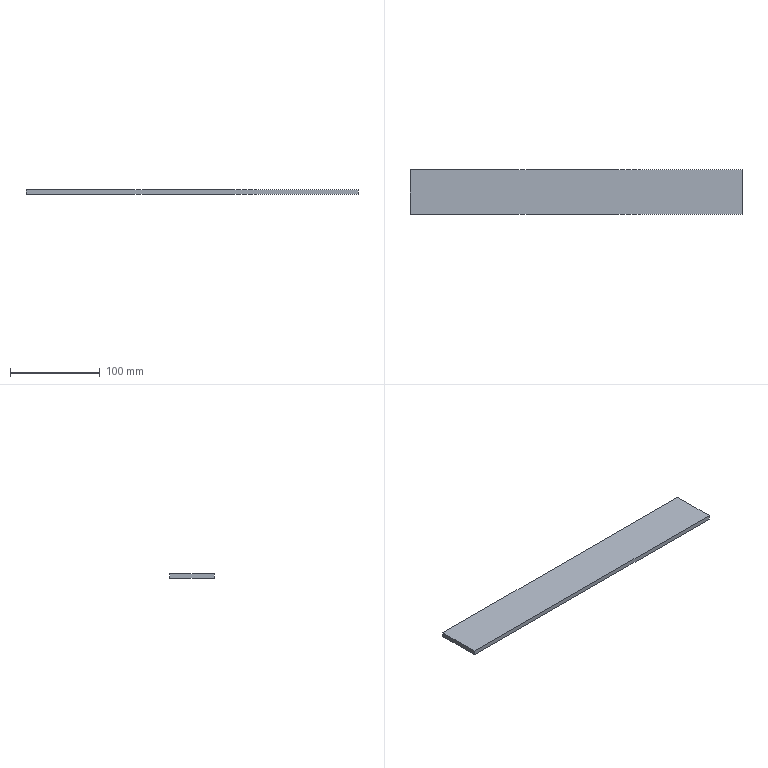Part | SolidWorks | features BaseBody 1 | 1 solid | 6 faces | box 370 x 50 x 5 mm | volume 92500 mm3 | plane 6
STEP:
#1=CARTESIAN_POINT('',(370.,50.,5.));
#2=VERTEX_POINT('',#1);
#3=CARTESIAN_POINT('',(0.,50.,5.));
#4=VERTEX_POINT('',#3);
#5=CARTESIAN_POINT('',(185.,50.,5.));
#6=DIRECTION('',(-1.,0.,0.));
#7=VECTOR('',#6,1000.);
#8=LINE('',#5,#7);
#9=EDGE_CURVE('',#2,#4,#8,.T.);
#10=ORIENTED_EDGE('',*,*,#9,.T.);
#11=CARTESIAN_POINT('',(0.,0.,5.));
#12=VERTEX_POINT('',#11);
#13=CARTESIAN_POINT('',(0.,25.,5.));
#14=DIRECTION('',(0.,-1.,0.));
#15=VECTOR('',#14,1000.);
#16=LINE('',#13,#15);
#17=EDGE_CURVE('',#4,#12,#16,.T.);
#18=ORIENTED_EDGE('',*,*,#17,.T.);
#19=CARTESIAN_POINT('',(370.,0.,5.));
#20=VERTEX_POINT('',#19);
#21=CARTESIAN_POINT('',(185.,0.,5.));
#22=DIRECTION('',(1.,0.,0.));
#23=VECTOR('',#22,1000.);
#24=LINE('',#21,#23);
#25=EDGE_CURVE('',#12,#20,#24,.T.);
#26=ORIENTED_EDGE('',*,*,#25,.T.);
#27=CARTESIAN_POINT('',(370.,25.,5.));
#28=DIRECTION('',(0.,1.,0.));
#29=VECTOR('',#28,1000.);
#30=LINE('',#27,#29);
#31=EDGE_CURVE('',#20,#2,#30,.T.);
#32=ORIENTED_EDGE('',*,*,#31,.T.);
#33=EDGE_LOOP('',(#10,#18,#26,#32));
#34=FACE_OUTER_BOUND('',#33,.T.);
#35=CARTESIAN_POINT('',(185.,25.,5.));
#36=DIRECTION('',(0.,0.,1.));
#37=DIRECTION('',(1.,0.,0.));
#38=AXIS2_PLACEMENT_3D('',#35,#36,#37);
#39=PLANE('',#38);
#40=ADVANCED_FACE('',(#34),#39,.T.);
#41=ORIENTED_EDGE('',*,*,#17,.F.);
#42=CARTESIAN_POINT('',(0.,50.,0.));
#43=VERTEX_POINT('',#42);
#44=CARTESIAN_POINT('',(0.,50.,0.));
#45=DIRECTION('',(0.,0.,-1.));
#46=VECTOR('',#45,1000.);
#47=LINE('',#44,#46);
#48=EDGE_CURVE('',#4,#43,#47,.T.);
#49=ORIENTED_EDGE('',*,*,#48,.T.);
#50=CARTESIAN_POINT('',(0.,0.,0.));
#51=VERTEX_POINT('',#50);
#52=CARTESIAN_POINT('',(0.,50.,0.));
#53=DIRECTION('',(0.,-1.,0.));
#54=VECTOR('',#53,1000.);
#55=LINE('',#52,#54);
#56=EDGE_CURVE('',#43,#51,#55,.T.);
#57=ORIENTED_EDGE('',*,*,#56,.T.);
#58=CARTESIAN_POINT('',(0.,0.,0.));
#59=DIRECTION('',(0.,0.,1.));
#60=VECTOR('',#59,1000.);
#61=LINE('',#58,#60);
#62=EDGE_CURVE('',#51,#12,#61,.T.);
#63=ORIENTED_EDGE('',*,*,#62,.T.);
#64=EDGE_LOOP('',(#41,#49,#57,#63));
#65=FACE_OUTER_BOUND('',#64,.T.);
#66=CARTESIAN_POINT('',(0.,50.,0.));
#67=DIRECTION('',(-1.,0.,0.));
#68=DIRECTION('',(0.,-1.,0.));
#69=AXIS2_PLACEMENT_3D('',#66,#67,#68);
#70=PLANE('',#69);
#71=ADVANCED_FACE('',(#65),#70,.T.);
#72=ORIENTED_EDGE('',*,*,#9,.F.);
#73=CARTESIAN_POINT('',(370.,50.,0.));
#74=VERTEX_POINT('',#73);
#75=CARTESIAN_POINT('',(370.,50.,0.));
#76=DIRECTION('',(0.,0.,-1.));
#77=VECTOR('',#76,1000.);
#78=LINE('',#75,#77);
#79=EDGE_CURVE('',#2,#74,#78,.T.);
#80=ORIENTED_EDGE('',*,*,#79,.T.);
#81=CARTESIAN_POINT('',(370.,50.,0.));
#82=DIRECTION('',(-1.,0.,0.));
#83=VECTOR('',#82,1000.);
#84=LINE('',#81,#83);
#85=EDGE_CURVE('',#74,#43,#84,.T.);
#86=ORIENTED_EDGE('',*,*,#85,.T.);
#87=ORIENTED_EDGE('',*,*,#48,.F.);
#88=EDGE_LOOP('',(#72,#80,#86,#87));
#89=FACE_OUTER_BOUND('',#88,.T.);
#90=CARTESIAN_POINT('',(370.,50.,0.));
#91=DIRECTION('',(0.,1.,0.));
#92=DIRECTION('',(-1.,0.,0.));
#93=AXIS2_PLACEMENT_3D('',#90,#91,#92);
#94=PLANE('',#93);
#95=ADVANCED_FACE('',(#89),#94,.T.);
#96=ORIENTED_EDGE('',*,*,#31,.F.);
#97=CARTESIAN_POINT('',(370.,0.,0.));
#98=VERTEX_POINT('',#97);
#99=CARTESIAN_POINT('',(370.,0.,0.));
#100=DIRECTION('',(0.,0.,-1.));
#101=VECTOR('',#100,1000.);
#102=LINE('',#99,#101);
#103=EDGE_CURVE('',#20,#98,#102,.T.);
#104=ORIENTED_EDGE('',*,*,#103,.T.);
#105=CARTESIAN_POINT('',(370.,0.,0.));
#106=DIRECTION('',(0.,1.,0.));
#107=VECTOR('',#106,1000.);
#108=LINE('',#105,#107);
#109=EDGE_CURVE('',#98,#74,#108,.T.);
#110=ORIENTED_EDGE('',*,*,#109,.T.);
#111=ORIENTED_EDGE('',*,*,#79,.F.);
#112=EDGE_LOOP('',(#96,#104,#110,#111));
#113=FACE_OUTER_BOUND('',#112,.T.);
#114=CARTESIAN_POINT('',(370.,0.,0.));
#115=DIRECTION('',(1.,0.,0.));
#116=DIRECTION('',(0.,0.,-1.));
#117=AXIS2_PLACEMENT_3D('',#114,#115,#116);
#118=PLANE('',#117);
#119=ADVANCED_FACE('',(#113),#118,.T.);
#120=ORIENTED_EDGE('',*,*,#25,.F.);
#121=ORIENTED_EDGE('',*,*,#62,.F.);
#122=CARTESIAN_POINT('',(0.,0.,0.));
#123=DIRECTION('',(1.,0.,0.));
#124=VECTOR('',#123,1000.);
#125=LINE('',#122,#124);
#126=EDGE_CURVE('',#51,#98,#125,.T.);
#127=ORIENTED_EDGE('',*,*,#126,.T.);
#128=ORIENTED_EDGE('',*,*,#103,.F.);
#129=EDGE_LOOP('',(#120,#121,#127,#128));
#130=FACE_OUTER_BOUND('',#129,.T.);
#131=CARTESIAN_POINT('',(0.,0.,0.));
#132=DIRECTION('',(0.,-1.,0.));
#133=DIRECTION('',(0.,0.,-1.));
#134=AXIS2_PLACEMENT_3D('',#131,#132,#133);
#135=PLANE('',#134);
#136=ADVANCED_FACE('',(#130),#135,.T.);
#137=ORIENTED_EDGE('',*,*,#56,.F.);
#138=ORIENTED_EDGE('',*,*,#85,.F.);
#139=ORIENTED_EDGE('',*,*,#109,.F.);
#140=ORIENTED_EDGE('',*,*,#126,.F.);
#141=EDGE_LOOP('',(#137,#138,#139,#140));
#142=FACE_OUTER_BOUND('',#141,.T.);
#143=CARTESIAN_POINT('',(185.,25.,0.));
#144=DIRECTION('',(0.,0.,1.));
#145=DIRECTION('',(1.,0.,0.));
#146=AXIS2_PLACEMENT_3D('',#143,#144,#145);
#147=PLANE('',#146);
#148=ADVANCED_FACE('',(#142),#147,.F.);
#149=CLOSED_SHELL('',(#40,#71,#95,#119,#136,#148));
#150=MANIFOLD_SOLID_BREP('',#149);
#151=CARTESIAN_POINT('',(0.,0.,0.));
#152=DIRECTION('',(0.,0.,1.));
#153=DIRECTION('',(1.,0.,0.));
#154=AXIS2_PLACEMENT_3D('',#151,#152,#153);
#155=(LENGTH_UNIT()NAMED_UNIT(*)SI_UNIT(.MILLI.,.METRE.));
#156=UNCERTAINTY_MEASURE_WITH_UNIT(LENGTH_MEASURE(0.00001),#155,'','');
#157=(NAMED_UNIT(*)PLANE_ANGLE_UNIT()SI_UNIT($,.RADIAN.));
#158=(NAMED_UNIT(*)SI_UNIT($,.STERADIAN.)SOLID_ANGLE_UNIT());
#159=(GEOMETRIC_REPRESENTATION_CONTEXT(3)GLOBAL_UNCERTAINTY_ASSIGNED_CONTEXT((#156))GLOBAL_UNIT_ASSIGNED_CONTEXT((#155,#157,#158))REPRESENTATION_CONTEXT('',''));
#160=ADVANCED_BREP_SHAPE_REPRESENTATION('',(#150,#154),#159);